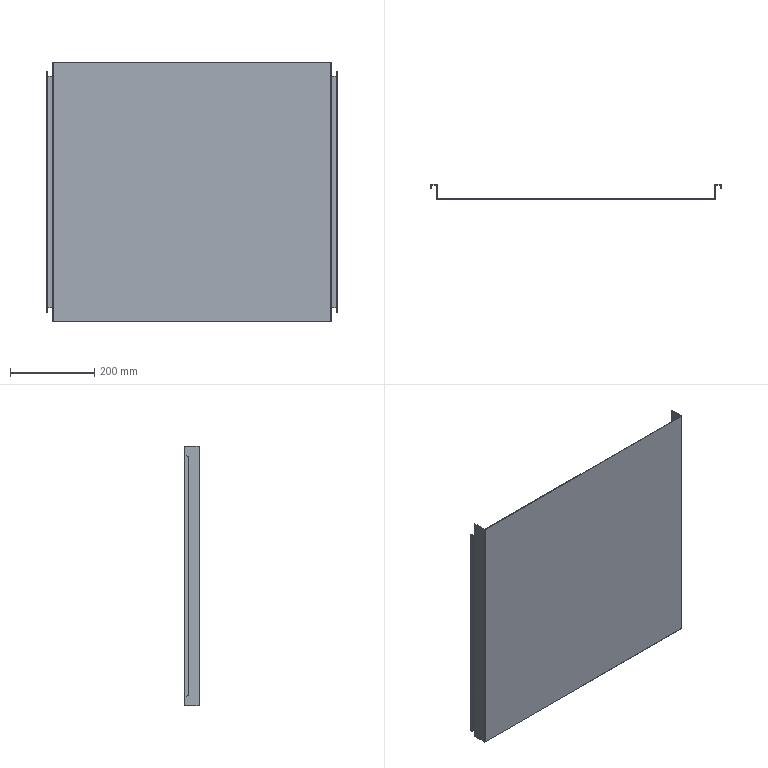Part | SolidWorks | features EdgeFlange 3, SMBaseFlange 3, Fillet 1, FlatPattern 1, SheetMetal 1 | 1 solid | 70 faces | box 689 x 36.5 x 617 mm | volume 712057 mm3 | plane 54 | cylinder 16 | commonest cylinder face diameters 0.2 x6 3.2 x6 10 x4